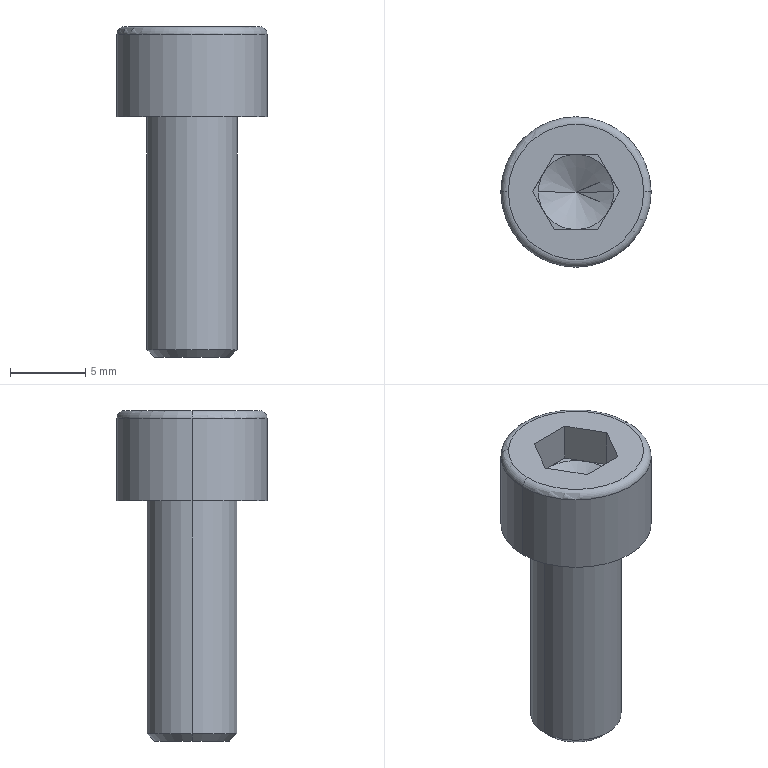Part | NX | features BREP 1 | 1 solid | 25 faces | box 10 x 10 x 22 mm | volume 854.017 mm3 | plane 15 | cone 4 | cylinder 4 | torus 2 | commonest cylinder face diameters 6 x2 10 x2
STEP:
#1=CARTESIAN_POINT('',(0.,0.,1.957));
#2=VERTEX_POINT('',#1);
#3=CARTESIAN_POINT('',(-2.5,0.,3.4));
#4=VERTEX_POINT('',#3);
#5=CARTESIAN_POINT('',(-2.5,0.,3.4));
#6=DIRECTION('',(-0.866,0.,0.5));
#7=VECTOR('',#6,1000.);
#8=LINE('',#5,#7);
#9=EDGE_CURVE('',#2,#4,#8,.T.);
#10=ORIENTED_EDGE('',*,*,#9,.F.);
#11=CARTESIAN_POINT('',(2.5,0.,3.4));
#12=VERTEX_POINT('',#11);
#13=CARTESIAN_POINT('',(2.5,0.,3.4));
#14=DIRECTION('',(0.866,0.,0.5));
#15=VECTOR('',#14,1000.);
#16=LINE('',#13,#15);
#17=EDGE_CURVE('',#2,#12,#16,.T.);
#18=ORIENTED_EDGE('',*,*,#17,.T.);
#19=CARTESIAN_POINT('',(2.165,1.25,3.4));
#20=VERTEX_POINT('',#19);
#21=CARTESIAN_POINT('',(0.,0.,3.4));
#22=DIRECTION('',(0.,0.,1.));
#23=DIRECTION('',(1.,0.,0.));
#24=AXIS2_PLACEMENT_3D('',#21,#22,#23);
#25=CIRCLE('',#24,2.5);
#26=EDGE_CURVE('',#12,#20,#25,.T.);
#27=ORIENTED_EDGE('',*,*,#26,.T.);
#28=CARTESIAN_POINT('',(0.,2.5,3.4));
#29=VERTEX_POINT('',#28);
#30=CARTESIAN_POINT('',(0.,0.,3.4));
#31=DIRECTION('',(0.,0.,1.));
#32=DIRECTION('',(1.,0.,0.));
#33=AXIS2_PLACEMENT_3D('',#30,#31,#32);
#34=CIRCLE('',#33,2.5);
#35=EDGE_CURVE('',#20,#29,#34,.T.);
#36=ORIENTED_EDGE('',*,*,#35,.T.);
#37=CARTESIAN_POINT('',(-2.165,1.25,3.4));
#38=VERTEX_POINT('',#37);
#39=CARTESIAN_POINT('',(0.,0.,3.4));
#40=DIRECTION('',(0.,0.,-1.));
#41=DIRECTION('',(-1.,0.,0.));
#42=AXIS2_PLACEMENT_3D('',#39,#40,#41);
#43=CIRCLE('',#42,2.5);
#44=EDGE_CURVE('',#38,#29,#43,.T.);
#45=ORIENTED_EDGE('',*,*,#44,.F.);
#46=CARTESIAN_POINT('',(0.,0.,3.4));
#47=DIRECTION('',(0.,0.,1.));
#48=DIRECTION('',(1.,0.,0.));
#49=AXIS2_PLACEMENT_3D('',#46,#47,#48);
#50=CIRCLE('',#49,2.5);
#51=EDGE_CURVE('',#38,#4,#50,.T.);
#52=ORIENTED_EDGE('',*,*,#51,.T.);
#53=EDGE_LOOP('',(#10,#18,#27,#36,#45,#52));
#54=FACE_BOUND('',#53,.T.);
#55=CARTESIAN_POINT('',(0.,0.,3.4));
#56=DIRECTION('',(0.,0.,1.));
#57=DIRECTION('',(-1.,0.,0.));
#58=AXIS2_PLACEMENT_3D('',#55,#56,#57);
#59=CONICAL_SURFACE('',#58,2.5,1.047);
#60=ADVANCED_FACE('',(#54),#59,.F.);
#61=CARTESIAN_POINT('',(-2.5,0.,-16.));
#62=VERTEX_POINT('',#61);
#63=CARTESIAN_POINT('',(2.5,0.,-16.));
#64=VERTEX_POINT('',#63);
#65=CARTESIAN_POINT('',(0.,0.,-16.));
#66=DIRECTION('',(0.,0.,1.));
#67=DIRECTION('',(-1.,0.,0.));
#68=AXIS2_PLACEMENT_3D('',#65,#66,#67);
#69=CIRCLE('',#68,2.5);
#70=EDGE_CURVE('',#62,#64,#69,.T.);
#71=ORIENTED_EDGE('',*,*,#70,.T.);
#72=CARTESIAN_POINT('',(3.,0.,-15.5));
#73=VERTEX_POINT('',#72);
#74=CARTESIAN_POINT('',(3.,0.,-15.5));
#75=DIRECTION('',(0.7071,0.,0.7071));
#76=VECTOR('',#75,1000.);
#77=LINE('',#74,#76);
#78=EDGE_CURVE('',#64,#73,#77,.T.);
#79=ORIENTED_EDGE('',*,*,#78,.T.);
#80=CARTESIAN_POINT('',(-3.,0.,-15.5));
#81=VERTEX_POINT('',#80);
#82=CARTESIAN_POINT('',(0.,0.,-15.5));
#83=DIRECTION('',(0.,0.,-1.));
#84=DIRECTION('',(-1.,0.,0.));
#85=AXIS2_PLACEMENT_3D('',#82,#83,#84);
#86=CIRCLE('',#85,3.);
#87=EDGE_CURVE('',#73,#81,#86,.T.);
#88=ORIENTED_EDGE('',*,*,#87,.T.);
#89=CARTESIAN_POINT('',(-3.,0.,-15.5));
#90=DIRECTION('',(-0.7071,0.,0.7071));
#91=VECTOR('',#90,1000.);
#92=LINE('',#89,#91);
#93=EDGE_CURVE('',#62,#81,#92,.T.);
#94=ORIENTED_EDGE('',*,*,#93,.F.);
#95=EDGE_LOOP('',(#71,#79,#88,#94));
#96=FACE_BOUND('',#95,.T.);
#97=CARTESIAN_POINT('',(0.,0.,-15.5));
#98=DIRECTION('',(0.,0.,1.));
#99=DIRECTION('',(-1.,0.,0.));
#100=AXIS2_PLACEMENT_3D('',#97,#98,#99);
#101=CONICAL_SURFACE('',#100,3.,0.7854);
#102=ADVANCED_FACE('',(#96),#101,.T.);
#103=CARTESIAN_POINT('',(4.5,0.,6.));
#104=VERTEX_POINT('',#103);
#105=CARTESIAN_POINT('',(-4.5,0.,6.));
#106=VERTEX_POINT('',#105);
#107=CARTESIAN_POINT('',(0.,0.,6.));
#108=DIRECTION('',(0.,0.,-1.));
#109=DIRECTION('',(1.,0.,0.));
#110=AXIS2_PLACEMENT_3D('',#107,#108,#109);
#111=CIRCLE('',#110,4.5);
#112=EDGE_CURVE('',#104,#106,#111,.T.);
#113=ORIENTED_EDGE('',*,*,#112,.T.);
#114=CARTESIAN_POINT('',(-5.,0.,5.5));
#115=VERTEX_POINT('',#114);
#116=CARTESIAN_POINT('',(-4.5,0.,5.5));
#117=DIRECTION('',(0.,-1.,0.));
#118=DIRECTION('',(1.,0.,0.));
#119=AXIS2_PLACEMENT_3D('',#116,#117,#118);
#120=CIRCLE('',#119,0.5);
#121=EDGE_CURVE('',#115,#106,#120,.F.);
#122=ORIENTED_EDGE('',*,*,#121,.F.);
#123=CARTESIAN_POINT('',(5.,0.,5.5));
#124=VERTEX_POINT('',#123);
#125=CARTESIAN_POINT('',(0.,0.,5.5));
#126=DIRECTION('',(0.,0.,1.));
#127=DIRECTION('',(1.,0.,0.));
#128=AXIS2_PLACEMENT_3D('',#125,#126,#127);
#129=CIRCLE('',#128,5.);
#130=EDGE_CURVE('',#115,#124,#129,.T.);
#131=ORIENTED_EDGE('',*,*,#130,.T.);
#132=CARTESIAN_POINT('',(4.5,0.,5.5));
#133=DIRECTION('',(0.,1.,0.));
#134=DIRECTION('',(0.,0.,1.));
#135=AXIS2_PLACEMENT_3D('',#132,#133,#134);
#136=CIRCLE('',#135,0.5);
#137=EDGE_CURVE('',#124,#104,#136,.F.);
#138=ORIENTED_EDGE('',*,*,#137,.T.);
#139=EDGE_LOOP('',(#113,#122,#131,#138));
#140=FACE_BOUND('',#139,.T.);
#141=CARTESIAN_POINT('',(0.,0.,5.5));
#142=DIRECTION('',(0.,0.,-1.));
#143=DIRECTION('',(1.,0.,0.));
#144=AXIS2_PLACEMENT_3D('',#141,#142,#143);
#145=TOROIDAL_SURFACE('',#144,4.5,0.5);
#146=ADVANCED_FACE('',(#140),#145,.T.);
#147=ORIENTED_EDGE('',*,*,#87,.F.);
#148=CARTESIAN_POINT('',(3.,0.,0.));
#149=VERTEX_POINT('',#148);
#150=CARTESIAN_POINT('',(3.,0.,-16.));
#151=DIRECTION('',(0.,0.,1.));
#152=VECTOR('',#151,1000.);
#153=LINE('',#150,#152);
#154=EDGE_CURVE('',#73,#149,#153,.T.);
#155=ORIENTED_EDGE('',*,*,#154,.T.);
#156=CARTESIAN_POINT('',(-3.,0.,0.));
#157=VERTEX_POINT('',#156);
#158=CARTESIAN_POINT('',(0.,0.,0.));
#159=DIRECTION('',(0.,0.,1.));
#160=DIRECTION('',(1.,0.,0.));
#161=AXIS2_PLACEMENT_3D('',#158,#159,#160);
#162=CIRCLE('',#161,3.);
#163=EDGE_CURVE('',#157,#149,#162,.T.);
#164=ORIENTED_EDGE('',*,*,#163,.F.);
#165=CARTESIAN_POINT('',(-3.,0.,-16.));
#166=DIRECTION('',(0.,0.,1.));
#167=VECTOR('',#166,1000.);
#168=LINE('',#165,#167);
#169=EDGE_CURVE('',#81,#157,#168,.T.);
#170=ORIENTED_EDGE('',*,*,#169,.F.);
#171=EDGE_LOOP('',(#147,#155,#164,#170));
#172=FACE_BOUND('',#171,.T.);
#173=CARTESIAN_POINT('',(0.,0.,-16.));
#174=DIRECTION('',(0.,0.,1.));
#175=DIRECTION('',(-1.,0.,0.));
#176=AXIS2_PLACEMENT_3D('',#173,#174,#175);
#177=CYLINDRICAL_SURFACE('',#176,3.);
#178=ADVANCED_FACE('',(#172),#177,.T.);
#179=ORIENTED_EDGE('',*,*,#130,.F.);
#180=CARTESIAN_POINT('',(-5.,0.,0.));
#181=VERTEX_POINT('',#180);
#182=CARTESIAN_POINT('',(-5.,0.,6.));
#183=DIRECTION('',(0.,0.,-1.));
#184=VECTOR('',#183,1000.);
#185=LINE('',#182,#184);
#186=EDGE_CURVE('',#181,#115,#185,.F.);
#187=ORIENTED_EDGE('',*,*,#186,.F.);
#188=CARTESIAN_POINT('',(5.,0.,0.));
#189=VERTEX_POINT('',#188);
#190=CARTESIAN_POINT('',(0.,0.,0.));
#191=DIRECTION('',(0.,0.,1.));
#192=DIRECTION('',(1.,0.,0.));
#193=AXIS2_PLACEMENT_3D('',#190,#191,#192);
#194=CIRCLE('',#193,5.);
#195=EDGE_CURVE('',#181,#189,#194,.T.);
#196=ORIENTED_EDGE('',*,*,#195,.T.);
#197=CARTESIAN_POINT('',(5.,0.,6.));
#198=DIRECTION('',(0.,0.,-1.));
#199=VECTOR('',#198,1000.);
#200=LINE('',#197,#199);
#201=EDGE_CURVE('',#189,#124,#200,.F.);
#202=ORIENTED_EDGE('',*,*,#201,.T.);
#203=EDGE_LOOP('',(#179,#187,#196,#202));
#204=FACE_BOUND('',#203,.T.);
#205=CARTESIAN_POINT('',(0.,0.,6.));
#206=DIRECTION('',(0.,0.,-1.));
#207=DIRECTION('',(1.,0.,0.));
#208=AXIS2_PLACEMENT_3D('',#205,#206,#207);
#209=CYLINDRICAL_SURFACE('',#208,5.);
#210=ADVANCED_FACE('',(#204),#209,.T.);
#211=CARTESIAN_POINT('',(1.443,2.5,3.4));
#212=VERTEX_POINT('',#211);
#213=CARTESIAN_POINT('',(2.887,0.,3.4));
#214=DIRECTION('',(-0.5,0.866,0.));
#215=VECTOR('',#214,1000.);
#216=LINE('',#213,#215);
#217=EDGE_CURVE('',#20,#212,#216,.T.);
#218=ORIENTED_EDGE('',*,*,#217,.T.);
#219=CARTESIAN_POINT('',(1.443,2.5,3.4));
#220=DIRECTION('',(-1.,0.,0.));
#221=VECTOR('',#220,1000.);
#222=LINE('',#219,#221);
#223=EDGE_CURVE('',#212,#29,#222,.T.);
#224=ORIENTED_EDGE('',*,*,#223,.T.);
#225=ORIENTED_EDGE('',*,*,#35,.F.);
#226=EDGE_LOOP('',(#218,#224,#225));
#227=FACE_BOUND('',#226,.T.);
#228=CARTESIAN_POINT('',(0.,0.,3.4));
#229=DIRECTION('',(0.,0.,-1.));
#230=DIRECTION('',(0.,-1.,0.));
#231=AXIS2_PLACEMENT_3D('',#228,#229,#230);
#232=PLANE('',#231);
#233=ADVANCED_FACE('',(#227),#232,.F.);
#234=CARTESIAN_POINT('',(-1.443,2.5,3.4));
#235=VERTEX_POINT('',#234);
#236=CARTESIAN_POINT('',(1.443,2.5,3.4));
#237=DIRECTION('',(-1.,0.,0.));
#238=VECTOR('',#237,1000.);
#239=LINE('',#236,#238);
#240=EDGE_CURVE('',#29,#235,#239,.T.);
#241=ORIENTED_EDGE('',*,*,#240,.T.);
#242=CARTESIAN_POINT('',(-1.443,2.5,3.4));
#243=DIRECTION('',(-0.5,-0.866,0.));
#244=VECTOR('',#243,1000.);
#245=LINE('',#242,#244);
#246=EDGE_CURVE('',#235,#38,#245,.T.);
#247=ORIENTED_EDGE('',*,*,#246,.T.);
#248=ORIENTED_EDGE('',*,*,#44,.T.);
#249=EDGE_LOOP('',(#241,#247,#248));
#250=FACE_BOUND('',#249,.T.);
#251=CARTESIAN_POINT('',(0.,0.,3.4));
#252=DIRECTION('',(0.,0.,-1.));
#253=DIRECTION('',(0.,-1.,0.));
#254=AXIS2_PLACEMENT_3D('',#251,#252,#253);
#255=PLANE('',#254);
#256=ADVANCED_FACE('',(#250),#255,.F.);
#257=CARTESIAN_POINT('',(-2.887,0.,3.4));
#258=VERTEX_POINT('',#257);
#259=CARTESIAN_POINT('',(-1.443,2.5,3.4));
#260=DIRECTION('',(-0.5,-0.866,0.));
#261=VECTOR('',#260,1000.);
#262=LINE('',#259,#261);
#263=EDGE_CURVE('',#38,#258,#262,.T.);
#264=ORIENTED_EDGE('',*,*,#263,.T.);
#265=CARTESIAN_POINT('',(-2.165,-1.25,3.4));
#266=VERTEX_POINT('',#265);
#267=CARTESIAN_POINT('',(-2.887,0.,3.4));
#268=DIRECTION('',(0.5,-0.866,0.));
#269=VECTOR('',#268,1000.);
#270=LINE('',#267,#269);
#271=EDGE_CURVE('',#258,#266,#270,.T.);
#272=ORIENTED_EDGE('',*,*,#271,.T.);
#273=CARTESIAN_POINT('',(0.,0.,3.4));
#274=DIRECTION('',(0.,0.,1.));
#275=DIRECTION('',(1.,0.,0.));
#276=AXIS2_PLACEMENT_3D('',#273,#274,#275);
#277=CIRCLE('',#276,2.5);
#278=EDGE_CURVE('',#4,#266,#277,.T.);
#279=ORIENTED_EDGE('',*,*,#278,.F.);
#280=ORIENTED_EDGE('',*,*,#51,.F.);
#281=EDGE_LOOP('',(#264,#272,#279,#280));
#282=FACE_BOUND('',#281,.T.);
#283=CARTESIAN_POINT('',(0.,0.,3.4));
#284=DIRECTION('',(0.,0.,-1.));
#285=DIRECTION('',(0.,-1.,0.));
#286=AXIS2_PLACEMENT_3D('',#283,#284,#285);
#287=PLANE('',#286);
#288=ADVANCED_FACE('',(#282),#287,.F.);
#289=CARTESIAN_POINT('',(-1.443,-2.5,3.4));
#290=VERTEX_POINT('',#289);
#291=CARTESIAN_POINT('',(-2.887,0.,3.4));
#292=DIRECTION('',(0.5,-0.866,0.));
#293=VECTOR('',#292,1000.);
#294=LINE('',#291,#293);
#295=EDGE_CURVE('',#266,#290,#294,.T.);
#296=ORIENTED_EDGE('',*,*,#295,.T.);
#297=CARTESIAN_POINT('',(0.,-2.5,3.4));
#298=VERTEX_POINT('',#297);
#299=CARTESIAN_POINT('',(-1.443,-2.5,3.4));
#300=DIRECTION('',(1.,0.,0.));
#301=VECTOR('',#300,1000.);
#302=LINE('',#299,#301);
#303=EDGE_CURVE('',#290,#298,#302,.T.);
#304=ORIENTED_EDGE('',*,*,#303,.T.);
#305=CARTESIAN_POINT('',(0.,0.,3.4));
#306=DIRECTION('',(0.,0.,1.));
#307=DIRECTION('',(1.,0.,0.));
#308=AXIS2_PLACEMENT_3D('',#305,#306,#307);
#309=CIRCLE('',#308,2.5);
#310=EDGE_CURVE('',#266,#298,#309,.T.);
#311=ORIENTED_EDGE('',*,*,#310,.F.);
#312=EDGE_LOOP('',(#296,#304,#311));
#313=FACE_BOUND('',#312,.T.);
#314=CARTESIAN_POINT('',(0.,0.,3.4));
#315=DIRECTION('',(0.,0.,-1.));
#316=DIRECTION('',(0.,-1.,0.));
#317=AXIS2_PLACEMENT_3D('',#314,#315,#316);
#318=PLANE('',#317);
#319=ADVANCED_FACE('',(#313),#318,.F.);
#320=CARTESIAN_POINT('',(1.443,-2.5,3.4));
#321=VERTEX_POINT('',#320);
#322=CARTESIAN_POINT('',(-1.443,-2.5,3.4));
#323=DIRECTION('',(1.,0.,0.));
#324=VECTOR('',#323,1000.);
#325=LINE('',#322,#324);
#326=EDGE_CURVE('',#298,#321,#325,.T.);
#327=ORIENTED_EDGE('',*,*,#326,.T.);
#328=CARTESIAN_POINT('',(2.165,-1.25,3.4));
#329=VERTEX_POINT('',#328);
#330=CARTESIAN_POINT('',(1.443,-2.5,3.4));
#331=DIRECTION('',(0.5,0.866,0.));
#332=VECTOR('',#331,1000.);
#333=LINE('',#330,#332);
#334=EDGE_CURVE('',#321,#329,#333,.T.);
#335=ORIENTED_EDGE('',*,*,#334,.T.);
#336=CARTESIAN_POINT('',(0.,0.,3.4));
#337=DIRECTION('',(0.,0.,1.));
#338=DIRECTION('',(1.,0.,0.));
#339=AXIS2_PLACEMENT_3D('',#336,#337,#338);
#340=CIRCLE('',#339,2.5);
#341=EDGE_CURVE('',#298,#329,#340,.T.);
#342=ORIENTED_EDGE('',*,*,#341,.F.);
#343=EDGE_LOOP('',(#327,#335,#342));
#344=FACE_BOUND('',#343,.T.);
#345=CARTESIAN_POINT('',(0.,0.,3.4));
#346=DIRECTION('',(0.,0.,-1.));
#347=DIRECTION('',(0.,-1.,0.));
#348=AXIS2_PLACEMENT_3D('',#345,#346,#347);
#349=PLANE('',#348);
#350=ADVANCED_FACE('',(#344),#349,.F.);
#351=ORIENTED_EDGE('',*,*,#112,.F.);
#352=CARTESIAN_POINT('',(0.,0.,6.));
#353=DIRECTION('',(0.,0.,-1.));
#354=DIRECTION('',(1.,0.,0.));
#355=AXIS2_PLACEMENT_3D('',#352,#353,#354);
#356=CIRCLE('',#355,4.5);
#357=EDGE_CURVE('',#106,#104,#356,.T.);
#358=ORIENTED_EDGE('',*,*,#357,.F.);
#359=EDGE_LOOP('',(#351,#358));
#360=FACE_BOUND('',#359,.T.);
#361=CARTESIAN_POINT('',(2.887,0.,6.));
#362=VERTEX_POINT('',#361);
#363=CARTESIAN_POINT('',(1.443,2.5,6.));
#364=VERTEX_POINT('',#363);
#365=CARTESIAN_POINT('',(2.887,0.,6.));
#366=DIRECTION('',(-0.5,0.866,0.));
#367=VECTOR('',#366,1000.);
#368=LINE('',#365,#367);
#369=EDGE_CURVE('',#362,#364,#368,.T.);
#370=ORIENTED_EDGE('',*,*,#369,.F.);
#371=CARTESIAN_POINT('',(1.443,-2.5,6.));
#372=VERTEX_POINT('',#371);
#373=CARTESIAN_POINT('',(1.443,-2.5,6.));
#374=DIRECTION('',(0.5,0.866,0.));
#375=VECTOR('',#374,1000.);
#376=LINE('',#373,#375);
#377=EDGE_CURVE('',#372,#362,#376,.T.);
#378=ORIENTED_EDGE('',*,*,#377,.F.);
#379=CARTESIAN_POINT('',(-1.443,-2.5,6.));
#380=VERTEX_POINT('',#379);
#381=CARTESIAN_POINT('',(-1.443,-2.5,6.));
#382=DIRECTION('',(1.,0.,0.));
#383=VECTOR('',#382,1000.);
#384=LINE('',#381,#383);
#385=EDGE_CURVE('',#380,#372,#384,.T.);
#386=ORIENTED_EDGE('',*,*,#385,.F.);
#387=CARTESIAN_POINT('',(-2.887,0.,6.));
#388=VERTEX_POINT('',#387);
#389=CARTESIAN_POINT('',(-2.887,0.,6.));
#390=DIRECTION('',(0.5,-0.866,0.));
#391=VECTOR('',#390,1000.);
#392=LINE('',#389,#391);
#393=EDGE_CURVE('',#388,#380,#392,.T.);
#394=ORIENTED_EDGE('',*,*,#393,.F.);
#395=CARTESIAN_POINT('',(-1.443,2.5,6.));
#396=VERTEX_POINT('',#395);
#397=CARTESIAN_POINT('',(-1.443,2.5,6.));
#398=DIRECTION('',(-0.5,-0.866,0.));
#399=VECTOR('',#398,1000.);
#400=LINE('',#397,#399);
#401=EDGE_CURVE('',#396,#388,#400,.T.);
#402=ORIENTED_EDGE('',*,*,#401,.F.);
#403=CARTESIAN_POINT('',(1.443,2.5,6.));
#404=DIRECTION('',(-1.,0.,0.));
#405=VECTOR('',#404,1000.);
#406=LINE('',#403,#405);
#407=EDGE_CURVE('',#364,#396,#406,.T.);
#408=ORIENTED_EDGE('',*,*,#407,.F.);
#409=EDGE_LOOP('',(#370,#378,#386,#394,#402,#408));
#410=FACE_BOUND('',#409,.T.);
#411=CARTESIAN_POINT('',(0.,0.,6.));
#412=DIRECTION('',(0.,0.,-1.));
#413=DIRECTION('',(0.,-1.,0.));
#414=AXIS2_PLACEMENT_3D('',#411,#412,#413);
#415=PLANE('',#414);
#416=ADVANCED_FACE('',(#360,#410),#415,.F.);
#417=ORIENTED_EDGE('',*,*,#186,.T.);
#418=CARTESIAN_POINT('',(0.,0.,5.5));
#419=DIRECTION('',(0.,0.,1.));
#420=DIRECTION('',(1.,0.,0.));
#421=AXIS2_PLACEMENT_3D('',#418,#419,#420);
#422=CIRCLE('',#421,5.);
#423=EDGE_CURVE('',#124,#115,#422,.T.);
#424=ORIENTED_EDGE('',*,*,#423,.F.);
#425=ORIENTED_EDGE('',*,*,#201,.F.);
#426=CARTESIAN_POINT('',(0.,0.,0.));
#427=DIRECTION('',(0.,0.,1.));
#428=DIRECTION('',(1.,0.,0.));
#429=AXIS2_PLACEMENT_3D('',#426,#427,#428);
#430=CIRCLE('',#429,5.);
#431=EDGE_CURVE('',#189,#181,#430,.T.);
#432=ORIENTED_EDGE('',*,*,#431,.T.);
#433=EDGE_LOOP('',(#417,#424,#425,#432));
#434=FACE_BOUND('',#433,.T.);
#435=CARTESIAN_POINT('',(0.,0.,6.));
#436=DIRECTION('',(0.,0.,-1.));
#437=DIRECTION('',(1.,0.,0.));
#438=AXIS2_PLACEMENT_3D('',#435,#436,#437);
#439=CYLINDRICAL_SURFACE('',#438,5.);
#440=ADVANCED_FACE('',(#434),#439,.T.);
#441=ORIENTED_EDGE('',*,*,#431,.F.);
#442=ORIENTED_EDGE('',*,*,#195,.F.);
#443=EDGE_LOOP('',(#441,#442));
#444=FACE_BOUND('',#443,.T.);
#445=ORIENTED_EDGE('',*,*,#163,.T.);
#446=CARTESIAN_POINT('',(0.,0.,0.));
#447=DIRECTION('',(0.,0.,1.));
#448=DIRECTION('',(1.,0.,0.));
#449=AXIS2_PLACEMENT_3D('',#446,#447,#448);
#450=CIRCLE('',#449,3.);
#451=EDGE_CURVE('',#149,#157,#450,.T.);
#452=ORIENTED_EDGE('',*,*,#451,.T.);
#453=EDGE_LOOP('',(#445,#452));
#454=FACE_BOUND('',#453,.T.);
#455=CARTESIAN_POINT('',(0.,0.,0.));
#456=DIRECTION('',(0.,0.,-1.));
#457=DIRECTION('',(0.,-1.,0.));
#458=AXIS2_PLACEMENT_3D('',#455,#456,#457);
#459=PLANE('',#458);
#460=ADVANCED_FACE('',(#444,#454),#459,.T.);
#461=ORIENTED_EDGE('',*,*,#154,.F.);
#462=CARTESIAN_POINT('',(0.,0.,-15.5));
#463=DIRECTION('',(0.,0.,-1.));
#464=DIRECTION('',(-1.,0.,0.));
#465=AXIS2_PLACEMENT_3D('',#462,#463,#464);
#466=CIRCLE('',#465,3.);
#467=EDGE_CURVE('',#81,#73,#466,.T.);
#468=ORIENTED_EDGE('',*,*,#467,.F.);
#469=ORIENTED_EDGE('',*,*,#169,.T.);
#470=ORIENTED_EDGE('',*,*,#451,.F.);
#471=EDGE_LOOP('',(#461,#468,#469,#470));
#472=FACE_BOUND('',#471,.T.);
#473=CARTESIAN_POINT('',(0.,0.,-16.));
#474=DIRECTION('',(0.,0.,1.));
#475=DIRECTION('',(-1.,0.,0.));
#476=AXIS2_PLACEMENT_3D('',#473,#474,#475);
#477=CYLINDRICAL_SURFACE('',#476,3.);
#478=ADVANCED_FACE('',(#472),#477,.T.);
#479=ORIENTED_EDGE('',*,*,#70,.F.);
#480=CARTESIAN_POINT('',(0.,0.,-16.));
#481=DIRECTION('',(0.,0.,1.));
#482=DIRECTION('',(-1.,0.,0.));
#483=AXIS2_PLACEMENT_3D('',#480,#481,#482);
#484=CIRCLE('',#483,2.5);
#485=EDGE_CURVE('',#64,#62,#484,.T.);
#486=ORIENTED_EDGE('',*,*,#485,.F.);
#487=EDGE_LOOP('',(#479,#486));
#488=FACE_BOUND('',#487,.T.);
#489=CARTESIAN_POINT('',(0.,0.,-16.));
#490=DIRECTION('',(0.,0.,1.));
#491=DIRECTION('',(1.,0.,0.));
#492=AXIS2_PLACEMENT_3D('',#489,#490,#491);
#493=PLANE('',#492);
#494=ADVANCED_FACE('',(#488),#493,.F.);
#495=ORIENTED_EDGE('',*,*,#121,.T.);
#496=ORIENTED_EDGE('',*,*,#357,.T.);
#497=ORIENTED_EDGE('',*,*,#137,.F.);
#498=ORIENTED_EDGE('',*,*,#423,.T.);
#499=EDGE_LOOP('',(#495,#496,#497,#498));
#500=FACE_BOUND('',#499,.T.);
#501=CARTESIAN_POINT('',(0.,0.,5.5));
#502=DIRECTION('',(0.,0.,-1.));
#503=DIRECTION('',(1.,0.,0.));
#504=AXIS2_PLACEMENT_3D('',#501,#502,#503);
#505=TOROIDAL_SURFACE('',#504,4.5,0.5);
#506=ADVANCED_FACE('',(#500),#505,.T.);
#507=ORIENTED_EDGE('',*,*,#78,.F.);
#508=ORIENTED_EDGE('',*,*,#485,.T.);
#509=ORIENTED_EDGE('',*,*,#93,.T.);
#510=ORIENTED_EDGE('',*,*,#467,.T.);
#511=EDGE_LOOP('',(#507,#508,#509,#510));
#512=FACE_BOUND('',#511,.T.);
#513=CARTESIAN_POINT('',(0.,0.,-15.5));
#514=DIRECTION('',(0.,0.,1.));
#515=DIRECTION('',(-1.,0.,0.));
#516=AXIS2_PLACEMENT_3D('',#513,#514,#515);
#517=CONICAL_SURFACE('',#516,3.,0.7854);
#518=ADVANCED_FACE('',(#512),#517,.T.);
#519=ORIENTED_EDGE('',*,*,#369,.T.);
#520=CARTESIAN_POINT('',(1.443,2.5,3.4));
#521=DIRECTION('',(0.,0.,1.));
#522=VECTOR('',#521,1000.);
#523=LINE('',#520,#522);
#524=EDGE_CURVE('',#212,#364,#523,.T.);
#525=ORIENTED_EDGE('',*,*,#524,.F.);
#526=ORIENTED_EDGE('',*,*,#217,.F.);
#527=CARTESIAN_POINT('',(2.887,0.,3.4));
#528=VERTEX_POINT('',#527);
#529=CARTESIAN_POINT('',(2.887,0.,3.4));
#530=DIRECTION('',(-0.5,0.866,0.));
#531=VECTOR('',#530,1000.);
#532=LINE('',#529,#531);
#533=EDGE_CURVE('',#528,#20,#532,.T.);
#534=ORIENTED_EDGE('',*,*,#533,.F.);
#535=CARTESIAN_POINT('',(2.887,0.,3.4));
#536=DIRECTION('',(0.,0.,1.));
#537=VECTOR('',#536,1000.);
#538=LINE('',#535,#537);
#539=EDGE_CURVE('',#528,#362,#538,.T.);
#540=ORIENTED_EDGE('',*,*,#539,.T.);
#541=EDGE_LOOP('',(#519,#525,#526,#534,#540));
#542=FACE_BOUND('',#541,.T.);
#543=CARTESIAN_POINT('',(2.887,0.,3.4));
#544=DIRECTION('',(-0.866,-0.5,0.));
#545=DIRECTION('',(-0.5,0.866,0.));
#546=AXIS2_PLACEMENT_3D('',#543,#544,#545);
#547=PLANE('',#546);
#548=ADVANCED_FACE('',(#542),#547,.T.);
#549=ORIENTED_EDGE('',*,*,#407,.T.);
#550=CARTESIAN_POINT('',(-1.443,2.5,3.4));
#551=DIRECTION('',(0.,0.,1.));
#552=VECTOR('',#551,1000.);
#553=LINE('',#550,#552);
#554=EDGE_CURVE('',#235,#396,#553,.T.);
#555=ORIENTED_EDGE('',*,*,#554,.F.);
#556=ORIENTED_EDGE('',*,*,#240,.F.);
#557=ORIENTED_EDGE('',*,*,#223,.F.);
#558=ORIENTED_EDGE('',*,*,#524,.T.);
#559=EDGE_LOOP('',(#549,#555,#556,#557,#558));
#560=FACE_BOUND('',#559,.T.);
#561=CARTESIAN_POINT('',(1.443,2.5,3.4));
#562=DIRECTION('',(0.,-1.,0.));
#563=DIRECTION('',(0.,0.,-1.));
#564=AXIS2_PLACEMENT_3D('',#561,#562,#563);
#565=PLANE('',#564);
#566=ADVANCED_FACE('',(#560),#565,.T.);
#567=ORIENTED_EDGE('',*,*,#401,.T.);
#568=CARTESIAN_POINT('',(-2.887,0.,3.4));
#569=DIRECTION('',(0.,0.,1.));
#570=VECTOR('',#569,1000.);
#571=LINE('',#568,#570);
#572=EDGE_CURVE('',#258,#388,#571,.T.);
#573=ORIENTED_EDGE('',*,*,#572,.F.);
#574=ORIENTED_EDGE('',*,*,#263,.F.);
#575=ORIENTED_EDGE('',*,*,#246,.F.);
#576=ORIENTED_EDGE('',*,*,#554,.T.);
#577=EDGE_LOOP('',(#567,#573,#574,#575,#576));
#578=FACE_BOUND('',#577,.T.);
#579=CARTESIAN_POINT('',(-1.443,2.5,3.4));
#580=DIRECTION('',(0.866,-0.5,0.));
#581=DIRECTION('',(0.,0.,-1.));
#582=AXIS2_PLACEMENT_3D('',#579,#580,#581);
#583=PLANE('',#582);
#584=ADVANCED_FACE('',(#578),#583,.T.);
#585=ORIENTED_EDGE('',*,*,#393,.T.);
#586=CARTESIAN_POINT('',(-1.443,-2.5,3.4));
#587=DIRECTION('',(0.,0.,1.));
#588=VECTOR('',#587,1000.);
#589=LINE('',#586,#588);
#590=EDGE_CURVE('',#290,#380,#589,.T.);
#591=ORIENTED_EDGE('',*,*,#590,.F.);
#592=ORIENTED_EDGE('',*,*,#295,.F.);
#593=ORIENTED_EDGE('',*,*,#271,.F.);
#594=ORIENTED_EDGE('',*,*,#572,.T.);
#595=EDGE_LOOP('',(#585,#591,#592,#593,#594));
#596=FACE_BOUND('',#595,.T.);
#597=CARTESIAN_POINT('',(-2.887,0.,3.4));
#598=DIRECTION('',(0.866,0.5,0.));
#599=DIRECTION('',(0.,0.,-1.));
#600=AXIS2_PLACEMENT_3D('',#597,#598,#599);
#601=PLANE('',#600);
#602=ADVANCED_FACE('',(#596),#601,.T.);
#603=ORIENTED_EDGE('',*,*,#385,.T.);
#604=CARTESIAN_POINT('',(1.443,-2.5,3.4));
#605=DIRECTION('',(0.,0.,1.));
#606=VECTOR('',#605,1000.);
#607=LINE('',#604,#606);
#608=EDGE_CURVE('',#321,#372,#607,.T.);
#609=ORIENTED_EDGE('',*,*,#608,.F.);
#610=ORIENTED_EDGE('',*,*,#326,.F.);
#611=ORIENTED_EDGE('',*,*,#303,.F.);
#612=ORIENTED_EDGE('',*,*,#590,.T.);
#613=EDGE_LOOP('',(#603,#609,#610,#611,#612));
#614=FACE_BOUND('',#613,.T.);
#615=CARTESIAN_POINT('',(-1.443,-2.5,3.4));
#616=DIRECTION('',(0.,1.,0.));
#617=DIRECTION('',(1.,0.,0.));
#618=AXIS2_PLACEMENT_3D('',#615,#616,#617);
#619=PLANE('',#618);
#620=ADVANCED_FACE('',(#614),#619,.T.);
#621=ORIENTED_EDGE('',*,*,#377,.T.);
#622=ORIENTED_EDGE('',*,*,#539,.F.);
#623=CARTESIAN_POINT('',(1.443,-2.5,3.4));
#624=DIRECTION('',(0.5,0.866,0.));
#625=VECTOR('',#624,1000.);
#626=LINE('',#623,#625);
#627=EDGE_CURVE('',#329,#528,#626,.T.);
#628=ORIENTED_EDGE('',*,*,#627,.F.);
#629=ORIENTED_EDGE('',*,*,#334,.F.);
#630=ORIENTED_EDGE('',*,*,#608,.T.);
#631=EDGE_LOOP('',(#621,#622,#628,#629,#630));
#632=FACE_BOUND('',#631,.T.);
#633=CARTESIAN_POINT('',(1.443,-2.5,3.4));
#634=DIRECTION('',(-0.866,0.5,0.));
#635=DIRECTION('',(0.,0.,1.));
#636=AXIS2_PLACEMENT_3D('',#633,#634,#635);
#637=PLANE('',#636);
#638=ADVANCED_FACE('',(#632),#637,.T.);
#639=ORIENTED_EDGE('',*,*,#627,.T.);
#640=ORIENTED_EDGE('',*,*,#533,.T.);
#641=ORIENTED_EDGE('',*,*,#26,.F.);
#642=CARTESIAN_POINT('',(0.,0.,3.4));
#643=DIRECTION('',(0.,0.,1.));
#644=DIRECTION('',(1.,0.,0.));
#645=AXIS2_PLACEMENT_3D('',#642,#643,#644);
#646=CIRCLE('',#645,2.5);
#647=EDGE_CURVE('',#329,#12,#646,.T.);
#648=ORIENTED_EDGE('',*,*,#647,.F.);
#649=EDGE_LOOP('',(#639,#640,#641,#648));
#650=FACE_BOUND('',#649,.T.);
#651=CARTESIAN_POINT('',(0.,0.,3.4));
#652=DIRECTION('',(0.,0.,-1.));
#653=DIRECTION('',(0.,-1.,0.));
#654=AXIS2_PLACEMENT_3D('',#651,#652,#653);
#655=PLANE('',#654);
#656=ADVANCED_FACE('',(#650),#655,.F.);
#657=ORIENTED_EDGE('',*,*,#17,.F.);
#658=ORIENTED_EDGE('',*,*,#9,.T.);
#659=ORIENTED_EDGE('',*,*,#278,.T.);
#660=ORIENTED_EDGE('',*,*,#310,.T.);
#661=ORIENTED_EDGE('',*,*,#341,.T.);
#662=ORIENTED_EDGE('',*,*,#647,.T.);
#663=EDGE_LOOP('',(#657,#658,#659,#660,#661,#662));
#664=FACE_BOUND('',#663,.T.);
#665=CARTESIAN_POINT('',(0.,0.,3.4));
#666=DIRECTION('',(0.,0.,1.));
#667=DIRECTION('',(-1.,0.,0.));
#668=AXIS2_PLACEMENT_3D('',#665,#666,#667);
#669=CONICAL_SURFACE('',#668,2.5,1.047);
#670=ADVANCED_FACE('',(#664),#669,.F.);
#671=CLOSED_SHELL('',(#60,#102,#146,#178,#210,#233,#256,#288,#319,#350,#416,#440,#460,#478,#494,#506,#518,#548,#566,#584,#602,#620,#638,#656,#670));
#672=MANIFOLD_SOLID_BREP('',#671);
#673=(LENGTH_UNIT()NAMED_UNIT(*)SI_UNIT(.MILLI.,.METRE.));
#674=UNCERTAINTY_MEASURE_WITH_UNIT(LENGTH_MEASURE(0.00001),#673,'','');
#675=(NAMED_UNIT(*)PLANE_ANGLE_UNIT()SI_UNIT($,.RADIAN.));
#676=(NAMED_UNIT(*)SI_UNIT($,.STERADIAN.)SOLID_ANGLE_UNIT());
#677=(GEOMETRIC_REPRESENTATION_CONTEXT(3)GLOBAL_UNCERTAINTY_ASSIGNED_CONTEXT((#674))GLOBAL_UNIT_ASSIGNED_CONTEXT((#673,#675,#676))REPRESENTATION_CONTEXT('',''));
#678=ADVANCED_BREP_SHAPE_REPRESENTATION('',(#672),#677);